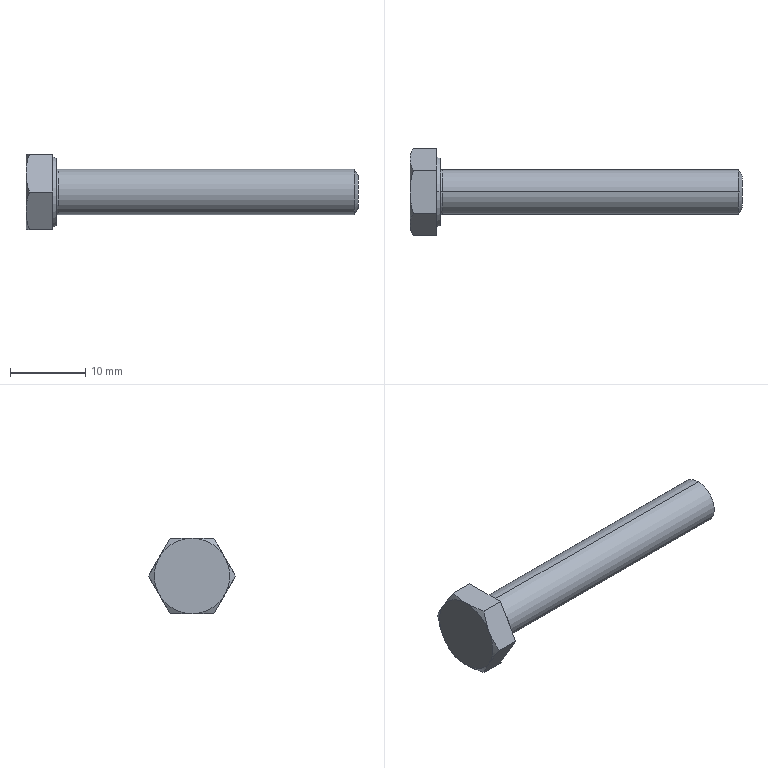Part | SolidWorks | features RevCut 3, Extrusion 1, Fillet 1, LPattern 1, Revolution 1 | 1 solid | 24 faces | box 44 x 11.547 x 10 mm | volume 1463 mm3 | cone 10 | plane 10 | torus 2 | cylinder 2 | commonest cylinder face diameters 6 x2
STEP:
#1=CARTESIAN_POINT('',(44.,0.,2.134));
#2=VERTEX_POINT('',#1);
#3=CARTESIAN_POINT('',(44.,0.,-2.134));
#4=VERTEX_POINT('',#3);
#5=CARTESIAN_POINT('',(44.,0.,0.));
#6=DIRECTION('',(-1.,0.,0.));
#7=DIRECTION('',(0.,0.,1.));
#8=AXIS2_PLACEMENT_3D('',#5,#6,#7);
#9=CIRCLE('',#8,2.134);
#10=EDGE_CURVE('',#2,#4,#9,.T.);
#11=ORIENTED_EDGE('',*,*,#10,.T.);
#12=CARTESIAN_POINT('',(43.5,0.,-3.));
#13=VERTEX_POINT('',#12);
#14=CARTESIAN_POINT('',(43.5,0.,-3.));
#15=DIRECTION('',(-0.5,0.,-0.866));
#16=VECTOR('',#15,1000.);
#17=LINE('',#14,#16);
#18=EDGE_CURVE('',#4,#13,#17,.T.);
#19=ORIENTED_EDGE('',*,*,#18,.T.);
#20=CARTESIAN_POINT('',(43.5,0.,3.));
#21=VERTEX_POINT('',#20);
#22=CARTESIAN_POINT('',(43.5,0.,0.));
#23=DIRECTION('',(-1.,0.,0.));
#24=DIRECTION('',(0.,0.,1.));
#25=AXIS2_PLACEMENT_3D('',#22,#23,#24);
#26=CIRCLE('',#25,3.);
#27=EDGE_CURVE('',#21,#13,#26,.T.);
#28=ORIENTED_EDGE('',*,*,#27,.F.);
#29=CARTESIAN_POINT('',(43.5,0.,3.));
#30=DIRECTION('',(-0.5,0.,0.866));
#31=VECTOR('',#30,1000.);
#32=LINE('',#29,#31);
#33=EDGE_CURVE('',#2,#21,#32,.T.);
#34=ORIENTED_EDGE('',*,*,#33,.F.);
#35=EDGE_LOOP('',(#11,#19,#28,#34));
#36=FACE_OUTER_BOUND('',#35,.T.);
#37=CARTESIAN_POINT('',(43.5,0.,0.));
#38=DIRECTION('',(-1.,0.,0.));
#39=DIRECTION('',(0.,0.,1.));
#40=AXIS2_PLACEMENT_3D('',#37,#38,#39);
#41=CONICAL_SURFACE('',#40,3.,1.047);
#42=ADVANCED_FACE('',(#36),#41,.T.);
#43=CARTESIAN_POINT('',(4.25,0.,3.));
#44=VERTEX_POINT('',#43);
#45=CARTESIAN_POINT('',(4.25,0.,-3.));
#46=VERTEX_POINT('',#45);
#47=CARTESIAN_POINT('',(4.25,0.,0.));
#48=DIRECTION('',(1.,0.,0.));
#49=DIRECTION('',(0.,0.,-1.));
#50=AXIS2_PLACEMENT_3D('',#47,#48,#49);
#51=CIRCLE('',#50,3.);
#52=EDGE_CURVE('',#44,#46,#51,.T.);
#53=ORIENTED_EDGE('',*,*,#52,.F.);
#54=CARTESIAN_POINT('',(4.,0.,3.25));
#55=VERTEX_POINT('',#54);
#56=CARTESIAN_POINT('',(4.25,0.,3.25));
#57=DIRECTION('',(0.,1.,0.));
#58=DIRECTION('',(0.,0.,1.));
#59=AXIS2_PLACEMENT_3D('',#56,#57,#58);
#60=CIRCLE('',#59,0.25);
#61=EDGE_CURVE('',#44,#55,#60,.T.);
#62=ORIENTED_EDGE('',*,*,#61,.T.);
#63=CARTESIAN_POINT('',(4.,0.,-3.25));
#64=VERTEX_POINT('',#63);
#65=CARTESIAN_POINT('',(4.,0.,0.));
#66=DIRECTION('',(-1.,0.,0.));
#67=DIRECTION('',(0.,0.,-1.));
#68=AXIS2_PLACEMENT_3D('',#65,#66,#67);
#69=CIRCLE('',#68,3.25);
#70=EDGE_CURVE('',#64,#55,#69,.T.);
#71=ORIENTED_EDGE('',*,*,#70,.F.);
#72=CARTESIAN_POINT('',(4.25,0.,-3.25));
#73=DIRECTION('',(0.,-1.,0.));
#74=DIRECTION('',(0.,0.,-1.));
#75=AXIS2_PLACEMENT_3D('',#72,#73,#74);
#76=CIRCLE('',#75,0.25);
#77=EDGE_CURVE('',#46,#64,#76,.T.);
#78=ORIENTED_EDGE('',*,*,#77,.F.);
#79=EDGE_LOOP('',(#53,#62,#71,#78));
#80=FACE_OUTER_BOUND('',#79,.T.);
#81=CARTESIAN_POINT('',(4.25,0.,0.));
#82=DIRECTION('',(1.,0.,0.));
#83=DIRECTION('',(0.,0.,-1.));
#84=AXIS2_PLACEMENT_3D('',#81,#82,#83);
#85=TOROIDAL_SURFACE('',#84,3.25,0.25);
#86=ADVANCED_FACE('',(#80),#85,.F.);
#87=CARTESIAN_POINT('',(4.,0.,4.44));
#88=VERTEX_POINT('',#87);
#89=CARTESIAN_POINT('',(4.,0.,-4.44));
#90=VERTEX_POINT('',#89);
#91=CARTESIAN_POINT('',(4.,0.,0.));
#92=DIRECTION('',(-1.,0.,0.));
#93=DIRECTION('',(0.,0.,1.));
#94=AXIS2_PLACEMENT_3D('',#91,#92,#93);
#95=CIRCLE('',#94,4.44);
#96=EDGE_CURVE('',#88,#90,#95,.T.);
#97=ORIENTED_EDGE('',*,*,#96,.T.);
#98=CARTESIAN_POINT('',(3.5,0.,-4.729));
#99=VERTEX_POINT('',#98);
#100=CARTESIAN_POINT('',(3.5,0.,-4.729));
#101=DIRECTION('',(-0.866,0.,-0.5));
#102=VECTOR('',#101,1000.);
#103=LINE('',#100,#102);
#104=EDGE_CURVE('',#90,#99,#103,.T.);
#105=ORIENTED_EDGE('',*,*,#104,.T.);
#106=CARTESIAN_POINT('',(3.5,0.,4.729));
#107=VERTEX_POINT('',#106);
#108=CARTESIAN_POINT('',(3.5,0.,0.));
#109=DIRECTION('',(-1.,0.,0.));
#110=DIRECTION('',(0.,0.,1.));
#111=AXIS2_PLACEMENT_3D('',#108,#109,#110);
#112=CIRCLE('',#111,4.729);
#113=EDGE_CURVE('',#107,#99,#112,.T.);
#114=ORIENTED_EDGE('',*,*,#113,.F.);
#115=CARTESIAN_POINT('',(3.5,0.,4.729));
#116=DIRECTION('',(-0.866,0.,0.5));
#117=VECTOR('',#116,1000.);
#118=LINE('',#115,#117);
#119=EDGE_CURVE('',#88,#107,#118,.T.);
#120=ORIENTED_EDGE('',*,*,#119,.F.);
#121=EDGE_LOOP('',(#97,#105,#114,#120));
#122=FACE_OUTER_BOUND('',#121,.T.);
#123=CARTESIAN_POINT('',(3.5,0.,0.));
#124=DIRECTION('',(-1.,0.,0.));
#125=DIRECTION('',(0.,0.,1.));
#126=AXIS2_PLACEMENT_3D('',#123,#124,#125);
#127=CONICAL_SURFACE('',#126,4.729,0.5236);
#128=ADVANCED_FACE('',(#122),#127,.T.);
#129=ORIENTED_EDGE('',*,*,#27,.T.);
#130=CARTESIAN_POINT('',(0.,0.,-3.));
#131=DIRECTION('',(-1.,0.,0.));
#132=VECTOR('',#131,1000.);
#133=LINE('',#130,#132);
#134=EDGE_CURVE('',#13,#46,#133,.T.);
#135=ORIENTED_EDGE('',*,*,#134,.T.);
#136=CARTESIAN_POINT('',(4.25,0.,0.));
#137=DIRECTION('',(1.,0.,0.));
#138=DIRECTION('',(0.,0.,-1.));
#139=AXIS2_PLACEMENT_3D('',#136,#137,#138);
#140=CIRCLE('',#139,3.);
#141=EDGE_CURVE('',#46,#44,#140,.T.);
#142=ORIENTED_EDGE('',*,*,#141,.T.);
#143=CARTESIAN_POINT('',(0.,0.,3.));
#144=DIRECTION('',(-1.,0.,0.));
#145=VECTOR('',#144,1000.);
#146=LINE('',#143,#145);
#147=EDGE_CURVE('',#21,#44,#146,.T.);
#148=ORIENTED_EDGE('',*,*,#147,.F.);
#149=EDGE_LOOP('',(#129,#135,#142,#148));
#150=FACE_OUTER_BOUND('',#149,.T.);
#151=CARTESIAN_POINT('',(0.,0.,0.));
#152=DIRECTION('',(-1.,0.,0.));
#153=DIRECTION('',(0.,0.,1.));
#154=AXIS2_PLACEMENT_3D('',#151,#152,#153);
#155=CYLINDRICAL_SURFACE('',#154,3.);
#156=ADVANCED_FACE('',(#150),#155,.T.);
#157=ORIENTED_EDGE('',*,*,#134,.F.);
#158=CARTESIAN_POINT('',(43.5,0.,0.));
#159=DIRECTION('',(-1.,0.,0.));
#160=DIRECTION('',(0.,0.,1.));
#161=AXIS2_PLACEMENT_3D('',#158,#159,#160);
#162=CIRCLE('',#161,3.);
#163=EDGE_CURVE('',#13,#21,#162,.T.);
#164=ORIENTED_EDGE('',*,*,#163,.T.);
#165=ORIENTED_EDGE('',*,*,#147,.T.);
#166=ORIENTED_EDGE('',*,*,#52,.T.);
#167=EDGE_LOOP('',(#157,#164,#165,#166));
#168=FACE_OUTER_BOUND('',#167,.T.);
#169=CARTESIAN_POINT('',(0.,0.,0.));
#170=DIRECTION('',(-1.,0.,0.));
#171=DIRECTION('',(0.,0.,1.));
#172=AXIS2_PLACEMENT_3D('',#169,#170,#171);
#173=CYLINDRICAL_SURFACE('',#172,3.);
#174=ADVANCED_FACE('',(#168),#173,.T.);
#175=CARTESIAN_POINT('',(3.5,2.887,-5.));
#176=VERTEX_POINT('',#175);
#177=CARTESIAN_POINT('',(3.5,5.774,0.));
#178=VERTEX_POINT('',#177);
#179=CARTESIAN_POINT('',(3.5,2.887,-5.));
#180=DIRECTION('',(0.,0.5,0.866));
#181=VECTOR('',#180,1000.);
#182=LINE('',#179,#181);
#183=EDGE_CURVE('',#176,#178,#182,.T.);
#184=ORIENTED_EDGE('',*,*,#183,.F.);
#185=CARTESIAN_POINT('',(0.4466,2.887,-5.));
#186=VERTEX_POINT('',#185);
#187=CARTESIAN_POINT('',(4.,2.887,-5.));
#188=DIRECTION('',(-1.,0.,0.));
#189=VECTOR('',#188,1000.);
#190=LINE('',#187,#189);
#191=EDGE_CURVE('',#176,#186,#190,.T.);
#192=ORIENTED_EDGE('',*,*,#191,.T.);
#193=CARTESIAN_POINT('',(0.,4.33,-2.5));
#194=VERTEX_POINT('',#193);
#195=CARTESIAN_POINT('',(0.,4.33,-2.5));
#196=CARTESIAN_POINT('',(0.,4.208,-2.712));
#197=CARTESIAN_POINT('',(0.01056,4.085,-2.925));
#198=CARTESIAN_POINT('',(0.0514,3.841,-3.347));
#199=CARTESIAN_POINT('',(0.08166,3.72,-3.556));
#200=CARTESIAN_POINT('',(0.1983,3.36,-4.181));
#201=CARTESIAN_POINT('',(0.3106,3.122,-4.592));
#202=CARTESIAN_POINT('',(0.4466,2.887,-5.));
#203=B_SPLINE_CURVE_WITH_KNOTS('',3,(#195,#196,#197,#198,#199,#200,#201,#202),.UNSPECIFIED.,.F.,.F.,(4,2,2,4),(0.002921,0.003649,0.004376,0.005831),.UNSPECIFIED.);
#204=EDGE_CURVE('',#194,#186,#203,.T.);
#205=ORIENTED_EDGE('',*,*,#204,.F.);
#206=CARTESIAN_POINT('',(0.4466,5.774,0.));
#207=VERTEX_POINT('',#206);
#208=CARTESIAN_POINT('',(0.4466,5.774,0.));
#209=CARTESIAN_POINT('',(0.1739,5.301,-0.8179));
#210=CARTESIAN_POINT('',(0.,4.822,-1.648));
#211=CARTESIAN_POINT('',(0.,4.33,-2.5));
#212=B_SPLINE_CURVE_WITH_KNOTS('',3,(#208,#209,#210,#211),.UNSPECIFIED.,.F.,.F.,(4,4),(0.000000238,0.002921),.UNSPECIFIED.);
#213=EDGE_CURVE('',#207,#194,#212,.T.);
#214=ORIENTED_EDGE('',*,*,#213,.F.);
#215=CARTESIAN_POINT('',(4.,5.774,0.));
#216=DIRECTION('',(-1.,0.,0.));
#217=VECTOR('',#216,1000.);
#218=LINE('',#215,#217);
#219=EDGE_CURVE('',#178,#207,#218,.T.);
#220=ORIENTED_EDGE('',*,*,#219,.F.);
#221=EDGE_LOOP('',(#184,#192,#205,#214,#220));
#222=FACE_OUTER_BOUND('',#221,.T.);
#223=CARTESIAN_POINT('',(4.,2.887,-5.));
#224=DIRECTION('',(0.,-0.866,0.5));
#225=DIRECTION('',(0.,-0.5,-0.866));
#226=AXIS2_PLACEMENT_3D('',#223,#224,#225);
#227=PLANE('',#226);
#228=ADVANCED_FACE('',(#222),#227,.F.);
#229=CARTESIAN_POINT('',(3.5,2.887,5.));
#230=VERTEX_POINT('',#229);
#231=CARTESIAN_POINT('',(3.5,5.774,0.));
#232=DIRECTION('',(0.,-0.5,0.866));
#233=VECTOR('',#232,1000.);
#234=LINE('',#231,#233);
#235=EDGE_CURVE('',#178,#230,#234,.T.);
#236=ORIENTED_EDGE('',*,*,#235,.F.);
#237=ORIENTED_EDGE('',*,*,#219,.T.);
#238=CARTESIAN_POINT('',(0.,4.33,2.5));
#239=VERTEX_POINT('',#238);
#240=CARTESIAN_POINT('',(0.,4.33,2.5));
#241=CARTESIAN_POINT('',(0.,4.453,2.288));
#242=CARTESIAN_POINT('',(0.01056,4.576,2.075));
#243=CARTESIAN_POINT('',(0.0514,4.819,1.653));
#244=CARTESIAN_POINT('',(0.08166,4.94,1.444));
#245=CARTESIAN_POINT('',(0.1983,5.3,0.8193));
#246=CARTESIAN_POINT('',(0.3106,5.538,0.4079));
#247=CARTESIAN_POINT('',(0.4466,5.774,0.));
#248=B_SPLINE_CURVE_WITH_KNOTS('',3,(#240,#241,#242,#243,#244,#245,#246,#247),.UNSPECIFIED.,.F.,.F.,(4,2,2,4),(0.002921,0.003649,0.004376,0.005831),.UNSPECIFIED.);
#249=EDGE_CURVE('',#239,#207,#248,.T.);
#250=ORIENTED_EDGE('',*,*,#249,.F.);
#251=CARTESIAN_POINT('',(0.4466,2.887,5.));
#252=VERTEX_POINT('',#251);
#253=CARTESIAN_POINT('',(0.4466,2.887,5.));
#254=CARTESIAN_POINT('',(0.1739,3.359,4.182));
#255=CARTESIAN_POINT('',(0.,3.838,3.352));
#256=CARTESIAN_POINT('',(0.,4.33,2.5));
#257=B_SPLINE_CURVE_WITH_KNOTS('',3,(#253,#254,#255,#256),.UNSPECIFIED.,.F.,.F.,(4,4),(0.000000238,0.002921),.UNSPECIFIED.);
#258=EDGE_CURVE('',#252,#239,#257,.T.);
#259=ORIENTED_EDGE('',*,*,#258,.F.);
#260=CARTESIAN_POINT('',(4.,2.887,5.));
#261=DIRECTION('',(-1.,0.,0.));
#262=VECTOR('',#261,1000.);
#263=LINE('',#260,#262);
#264=EDGE_CURVE('',#230,#252,#263,.T.);
#265=ORIENTED_EDGE('',*,*,#264,.F.);
#266=EDGE_LOOP('',(#236,#237,#250,#259,#265));
#267=FACE_OUTER_BOUND('',#266,.T.);
#268=CARTESIAN_POINT('',(4.,5.774,0.));
#269=DIRECTION('',(0.,-0.866,-0.5));
#270=DIRECTION('',(0.,0.5,-0.866));
#271=AXIS2_PLACEMENT_3D('',#268,#269,#270);
#272=PLANE('',#271);
#273=ADVANCED_FACE('',(#267),#272,.F.);
#274=CARTESIAN_POINT('',(3.5,-2.887,5.));
#275=VERTEX_POINT('',#274);
#276=CARTESIAN_POINT('',(3.5,2.887,5.));
#277=DIRECTION('',(0.,-1.,0.));
#278=VECTOR('',#277,1000.);
#279=LINE('',#276,#278);
#280=EDGE_CURVE('',#230,#275,#279,.T.);
#281=ORIENTED_EDGE('',*,*,#280,.F.);
#282=ORIENTED_EDGE('',*,*,#264,.T.);
#283=CARTESIAN_POINT('',(0.,0.,5.));
#284=VERTEX_POINT('',#283);
#285=CARTESIAN_POINT('',(0.,0.,5.));
#286=CARTESIAN_POINT('',(0.,0.4887,5.));
#287=CARTESIAN_POINT('',(0.04321,0.9837,5.));
#288=CARTESIAN_POINT('',(0.1996,1.947,5.));
#289=CARTESIAN_POINT('',(0.3118,2.42,5.));
#290=CARTESIAN_POINT('',(0.4466,2.887,5.));
#291=B_SPLINE_CURVE_WITH_KNOTS('',3,(#285,#286,#287,#288,#289,#290),.UNSPECIFIED.,.F.,.F.,(4,2,4),(0.008262,0.009724,0.01119),.UNSPECIFIED.);
#292=EDGE_CURVE('',#284,#252,#291,.T.);
#293=ORIENTED_EDGE('',*,*,#292,.F.);
#294=CARTESIAN_POINT('',(0.4466,-2.887,5.));
#295=VERTEX_POINT('',#294);
#296=CARTESIAN_POINT('',(0.4466,-2.887,5.));
#297=CARTESIAN_POINT('',(0.3109,-2.417,5.));
#298=CARTESIAN_POINT('',(0.1973,-1.936,5.));
#299=CARTESIAN_POINT('',(0.04202,-0.9731,5.));
#300=CARTESIAN_POINT('',(0.,-0.4884,5.));
#301=CARTESIAN_POINT('',(0.,0.,5.));
#302=B_SPLINE_CURVE_WITH_KNOTS('',3,(#296,#297,#298,#299,#300,#301),.UNSPECIFIED.,.F.,.F.,(4,2,4),(0.00534,0.006801,0.008262),.UNSPECIFIED.);
#303=EDGE_CURVE('',#295,#284,#302,.T.);
#304=ORIENTED_EDGE('',*,*,#303,.F.);
#305=CARTESIAN_POINT('',(4.,-2.887,5.));
#306=DIRECTION('',(-1.,0.,0.));
#307=VECTOR('',#306,1000.);
#308=LINE('',#305,#307);
#309=EDGE_CURVE('',#275,#295,#308,.T.);
#310=ORIENTED_EDGE('',*,*,#309,.F.);
#311=EDGE_LOOP('',(#281,#282,#293,#304,#310));
#312=FACE_OUTER_BOUND('',#311,.T.);
#313=CARTESIAN_POINT('',(4.,2.887,5.));
#314=DIRECTION('',(0.,0.,-1.));
#315=DIRECTION('',(0.,1.,0.));
#316=AXIS2_PLACEMENT_3D('',#313,#314,#315);
#317=PLANE('',#316);
#318=ADVANCED_FACE('',(#312),#317,.F.);
#319=CARTESIAN_POINT('',(3.5,-5.774,0.));
#320=VERTEX_POINT('',#319);
#321=CARTESIAN_POINT('',(3.5,-5.774,0.));
#322=DIRECTION('',(0.,-0.5,-0.866));
#323=VECTOR('',#322,1000.);
#324=LINE('',#321,#323);
#325=EDGE_CURVE('',#275,#320,#324,.T.);
#326=ORIENTED_EDGE('',*,*,#325,.F.);
#327=ORIENTED_EDGE('',*,*,#309,.T.);
#328=CARTESIAN_POINT('',(0.,-4.33,2.5));
#329=VERTEX_POINT('',#328);
#330=CARTESIAN_POINT('',(0.,-4.33,2.5));
#331=CARTESIAN_POINT('',(0.,-4.208,2.712));
#332=CARTESIAN_POINT('',(0.01056,-4.085,2.925));
#333=CARTESIAN_POINT('',(0.0514,-3.841,3.347));
#334=CARTESIAN_POINT('',(0.08166,-3.72,3.556));
#335=CARTESIAN_POINT('',(0.1983,-3.36,4.181));
#336=CARTESIAN_POINT('',(0.3106,-3.122,4.592));
#337=CARTESIAN_POINT('',(0.4466,-2.887,5.));
#338=B_SPLINE_CURVE_WITH_KNOTS('',3,(#330,#331,#332,#333,#334,#335,#336,#337),.UNSPECIFIED.,.F.,.F.,(4,2,2,4),(0.002921,0.003649,0.004376,0.005831),.UNSPECIFIED.);
#339=EDGE_CURVE('',#329,#295,#338,.T.);
#340=ORIENTED_EDGE('',*,*,#339,.F.);
#341=CARTESIAN_POINT('',(0.4466,-5.774,0.));
#342=VERTEX_POINT('',#341);
#343=CARTESIAN_POINT('',(0.4466,-5.774,0.));
#344=CARTESIAN_POINT('',(0.1739,-5.301,0.8179));
#345=CARTESIAN_POINT('',(0.,-4.822,1.648));
#346=CARTESIAN_POINT('',(0.,-4.33,2.5));
#347=B_SPLINE_CURVE_WITH_KNOTS('',3,(#343,#344,#345,#346),.UNSPECIFIED.,.F.,.F.,(4,4),(0.000000238,0.002921),.UNSPECIFIED.);
#348=EDGE_CURVE('',#342,#329,#347,.T.);
#349=ORIENTED_EDGE('',*,*,#348,.F.);
#350=CARTESIAN_POINT('',(4.,-5.774,0.));
#351=DIRECTION('',(-1.,0.,0.));
#352=VECTOR('',#351,1000.);
#353=LINE('',#350,#352);
#354=EDGE_CURVE('',#320,#342,#353,.T.);
#355=ORIENTED_EDGE('',*,*,#354,.F.);
#356=EDGE_LOOP('',(#326,#327,#340,#349,#355));
#357=FACE_OUTER_BOUND('',#356,.T.);
#358=CARTESIAN_POINT('',(4.,-5.774,0.));
#359=DIRECTION('',(0.,0.866,-0.5));
#360=DIRECTION('',(0.,0.5,0.866));
#361=AXIS2_PLACEMENT_3D('',#358,#359,#360);
#362=PLANE('',#361);
#363=ADVANCED_FACE('',(#357),#362,.F.);
#364=CARTESIAN_POINT('',(3.5,-2.887,-5.));
#365=VERTEX_POINT('',#364);
#366=CARTESIAN_POINT('',(3.5,-2.887,-5.));
#367=DIRECTION('',(0.,0.5,-0.866));
#368=VECTOR('',#367,1000.);
#369=LINE('',#366,#368);
#370=EDGE_CURVE('',#320,#365,#369,.T.);
#371=ORIENTED_EDGE('',*,*,#370,.F.);
#372=ORIENTED_EDGE('',*,*,#354,.T.);
#373=CARTESIAN_POINT('',(0.,-4.33,-2.5));
#374=VERTEX_POINT('',#373);
#375=CARTESIAN_POINT('',(0.,-4.33,-2.5));
#376=CARTESIAN_POINT('',(0.,-4.453,-2.288));
#377=CARTESIAN_POINT('',(0.01056,-4.576,-2.075));
#378=CARTESIAN_POINT('',(0.0514,-4.819,-1.653));
#379=CARTESIAN_POINT('',(0.08166,-4.94,-1.444));
#380=CARTESIAN_POINT('',(0.1983,-5.3,-0.8193));
#381=CARTESIAN_POINT('',(0.3106,-5.538,-0.4079));
#382=CARTESIAN_POINT('',(0.4466,-5.774,0.));
#383=B_SPLINE_CURVE_WITH_KNOTS('',3,(#375,#376,#377,#378,#379,#380,#381,#382),.UNSPECIFIED.,.F.,.F.,(4,2,2,4),(0.002921,0.003649,0.004376,0.005831),.UNSPECIFIED.);
#384=EDGE_CURVE('',#374,#342,#383,.T.);
#385=ORIENTED_EDGE('',*,*,#384,.F.);
#386=CARTESIAN_POINT('',(0.4466,-2.887,-5.));
#387=VERTEX_POINT('',#386);
#388=CARTESIAN_POINT('',(0.4466,-2.887,-5.));
#389=CARTESIAN_POINT('',(0.1739,-3.359,-4.182));
#390=CARTESIAN_POINT('',(0.,-3.838,-3.352));
#391=CARTESIAN_POINT('',(0.,-4.33,-2.5));
#392=B_SPLINE_CURVE_WITH_KNOTS('',3,(#388,#389,#390,#391),.UNSPECIFIED.,.F.,.F.,(4,4),(0.000000238,0.002921),.UNSPECIFIED.);
#393=EDGE_CURVE('',#387,#374,#392,.T.);
#394=ORIENTED_EDGE('',*,*,#393,.F.);
#395=CARTESIAN_POINT('',(4.,-2.887,-5.));
#396=DIRECTION('',(-1.,0.,0.));
#397=VECTOR('',#396,1000.);
#398=LINE('',#395,#397);
#399=EDGE_CURVE('',#365,#387,#398,.T.);
#400=ORIENTED_EDGE('',*,*,#399,.F.);
#401=EDGE_LOOP('',(#371,#372,#385,#394,#400));
#402=FACE_OUTER_BOUND('',#401,.T.);
#403=CARTESIAN_POINT('',(4.,-2.887,-5.));
#404=DIRECTION('',(0.,0.866,0.5));
#405=DIRECTION('',(0.,-0.5,0.866));
#406=AXIS2_PLACEMENT_3D('',#403,#404,#405);
#407=PLANE('',#406);
#408=ADVANCED_FACE('',(#402),#407,.F.);
#409=CARTESIAN_POINT('',(3.5,2.887,-5.));
#410=DIRECTION('',(0.,1.,0.));
#411=VECTOR('',#410,1000.);
#412=LINE('',#409,#411);
#413=EDGE_CURVE('',#365,#176,#412,.T.);
#414=ORIENTED_EDGE('',*,*,#413,.F.);
#415=ORIENTED_EDGE('',*,*,#399,.T.);
#416=CARTESIAN_POINT('',(0.,0.,-5.));
#417=VERTEX_POINT('',#416);
#418=CARTESIAN_POINT('',(0.,0.,-5.));
#419=CARTESIAN_POINT('',(0.,-0.4884,-5.));
#420=CARTESIAN_POINT('',(0.04202,-0.9731,-5.));
#421=CARTESIAN_POINT('',(0.1973,-1.936,-5.));
#422=CARTESIAN_POINT('',(0.3109,-2.417,-5.));
#423=CARTESIAN_POINT('',(0.4466,-2.887,-5.));
#424=B_SPLINE_CURVE_WITH_KNOTS('',3,(#418,#419,#420,#421,#422,#423),.UNSPECIFIED.,.F.,.F.,(4,2,4),(0.01799,0.01945,0.02091),.UNSPECIFIED.);
#425=EDGE_CURVE('',#417,#387,#424,.T.);
#426=ORIENTED_EDGE('',*,*,#425,.F.);
#427=CARTESIAN_POINT('',(0.4466,2.887,-5.));
#428=CARTESIAN_POINT('',(0.3118,2.42,-5.));
#429=CARTESIAN_POINT('',(0.1996,1.947,-5.));
#430=CARTESIAN_POINT('',(0.04321,0.9837,-5.));
#431=CARTESIAN_POINT('',(0.,0.4887,-5.));
#432=CARTESIAN_POINT('',(0.,0.,-5.));
#433=B_SPLINE_CURVE_WITH_KNOTS('',3,(#427,#428,#429,#430,#431,#432),.UNSPECIFIED.,.F.,.F.,(4,2,4),(0.01507,0.01653,0.01799),.UNSPECIFIED.);
#434=EDGE_CURVE('',#186,#417,#433,.T.);
#435=ORIENTED_EDGE('',*,*,#434,.F.);
#436=ORIENTED_EDGE('',*,*,#191,.F.);
#437=EDGE_LOOP('',(#414,#415,#426,#435,#436));
#438=FACE_OUTER_BOUND('',#437,.T.);
#439=CARTESIAN_POINT('',(4.,2.887,-5.));
#440=DIRECTION('',(0.,0.,1.));
#441=DIRECTION('',(0.,-1.,0.));
#442=AXIS2_PLACEMENT_3D('',#439,#440,#441);
#443=PLANE('',#442);
#444=ADVANCED_FACE('',(#438),#443,.F.);
#445=ORIENTED_EDGE('',*,*,#393,.T.);
#446=CARTESIAN_POINT('',(0.,0.,0.));
#447=DIRECTION('',(1.,0.,0.));
#448=DIRECTION('',(0.,0.,-1.));
#449=AXIS2_PLACEMENT_3D('',#446,#447,#448);
#450=CIRCLE('',#449,5.);
#451=EDGE_CURVE('',#374,#417,#450,.T.);
#452=ORIENTED_EDGE('',*,*,#451,.T.);
#453=ORIENTED_EDGE('',*,*,#425,.T.);
#454=EDGE_LOOP('',(#445,#452,#453));
#455=FACE_OUTER_BOUND('',#454,.T.);
#456=CARTESIAN_POINT('',(0.,0.,0.));
#457=DIRECTION('',(1.,0.,0.));
#458=DIRECTION('',(0.,0.,-1.));
#459=AXIS2_PLACEMENT_3D('',#456,#457,#458);
#460=CONICAL_SURFACE('',#459,5.,1.047);
#461=ADVANCED_FACE('',(#455),#460,.T.);
#462=ORIENTED_EDGE('',*,*,#348,.T.);
#463=CARTESIAN_POINT('',(0.,0.,0.));
#464=DIRECTION('',(1.,0.,0.));
#465=DIRECTION('',(0.,0.,-1.));
#466=AXIS2_PLACEMENT_3D('',#463,#464,#465);
#467=CIRCLE('',#466,5.);
#468=EDGE_CURVE('',#329,#374,#467,.T.);
#469=ORIENTED_EDGE('',*,*,#468,.T.);
#470=ORIENTED_EDGE('',*,*,#384,.T.);
#471=EDGE_LOOP('',(#462,#469,#470));
#472=FACE_OUTER_BOUND('',#471,.T.);
#473=CARTESIAN_POINT('',(0.,0.,0.));
#474=DIRECTION('',(1.,0.,0.));
#475=DIRECTION('',(0.,0.,-1.));
#476=AXIS2_PLACEMENT_3D('',#473,#474,#475);
#477=CONICAL_SURFACE('',#476,5.,1.047);
#478=ADVANCED_FACE('',(#472),#477,.T.);
#479=ORIENTED_EDGE('',*,*,#303,.T.);
#480=CARTESIAN_POINT('',(0.,0.,0.));
#481=DIRECTION('',(1.,0.,0.));
#482=DIRECTION('',(0.,0.,-1.));
#483=AXIS2_PLACEMENT_3D('',#480,#481,#482);
#484=CIRCLE('',#483,5.);
#485=EDGE_CURVE('',#284,#329,#484,.T.);
#486=ORIENTED_EDGE('',*,*,#485,.T.);
#487=ORIENTED_EDGE('',*,*,#339,.T.);
#488=EDGE_LOOP('',(#479,#486,#487));
#489=FACE_OUTER_BOUND('',#488,.T.);
#490=CARTESIAN_POINT('',(0.,0.,0.));
#491=DIRECTION('',(1.,0.,0.));
#492=DIRECTION('',(0.,0.,-1.));
#493=AXIS2_PLACEMENT_3D('',#490,#491,#492);
#494=CONICAL_SURFACE('',#493,5.,1.047);
#495=ADVANCED_FACE('',(#489),#494,.T.);
#496=ORIENTED_EDGE('',*,*,#292,.T.);
#497=ORIENTED_EDGE('',*,*,#258,.T.);
#498=CARTESIAN_POINT('',(0.,0.,0.));
#499=DIRECTION('',(-1.,0.,0.));
#500=DIRECTION('',(0.,0.,1.));
#501=AXIS2_PLACEMENT_3D('',#498,#499,#500);
#502=CIRCLE('',#501,5.);
#503=EDGE_CURVE('',#284,#239,#502,.T.);
#504=ORIENTED_EDGE('',*,*,#503,.F.);
#505=EDGE_LOOP('',(#496,#497,#504));
#506=FACE_OUTER_BOUND('',#505,.T.);
#507=CARTESIAN_POINT('',(0.,0.,0.));
#508=DIRECTION('',(1.,0.,0.));
#509=DIRECTION('',(0.,0.,-1.));
#510=AXIS2_PLACEMENT_3D('',#507,#508,#509);
#511=CONICAL_SURFACE('',#510,5.,1.047);
#512=ADVANCED_FACE('',(#506),#511,.T.);
#513=ORIENTED_EDGE('',*,*,#249,.T.);
#514=ORIENTED_EDGE('',*,*,#213,.T.);
#515=CARTESIAN_POINT('',(0.,0.,0.));
#516=DIRECTION('',(1.,0.,0.));
#517=DIRECTION('',(0.,0.,-1.));
#518=AXIS2_PLACEMENT_3D('',#515,#516,#517);
#519=CIRCLE('',#518,5.);
#520=EDGE_CURVE('',#194,#239,#519,.T.);
#521=ORIENTED_EDGE('',*,*,#520,.T.);
#522=EDGE_LOOP('',(#513,#514,#521));
#523=FACE_OUTER_BOUND('',#522,.T.);
#524=CARTESIAN_POINT('',(0.,0.,0.));
#525=DIRECTION('',(1.,0.,0.));
#526=DIRECTION('',(0.,0.,-1.));
#527=AXIS2_PLACEMENT_3D('',#524,#525,#526);
#528=CONICAL_SURFACE('',#527,5.,1.047);
#529=ADVANCED_FACE('',(#523),#528,.T.);
#530=ORIENTED_EDGE('',*,*,#204,.T.);
#531=ORIENTED_EDGE('',*,*,#434,.T.);
#532=CARTESIAN_POINT('',(0.,0.,0.));
#533=DIRECTION('',(1.,0.,0.));
#534=DIRECTION('',(0.,0.,-1.));
#535=AXIS2_PLACEMENT_3D('',#532,#533,#534);
#536=CIRCLE('',#535,5.);
#537=EDGE_CURVE('',#417,#194,#536,.T.);
#538=ORIENTED_EDGE('',*,*,#537,.T.);
#539=EDGE_LOOP('',(#530,#531,#538));
#540=FACE_OUTER_BOUND('',#539,.T.);
#541=CARTESIAN_POINT('',(0.,0.,0.));
#542=DIRECTION('',(1.,0.,0.));
#543=DIRECTION('',(0.,0.,-1.));
#544=AXIS2_PLACEMENT_3D('',#541,#542,#543);
#545=CONICAL_SURFACE('',#544,5.,1.047);
#546=ADVANCED_FACE('',(#540),#545,.T.);
#547=ORIENTED_EDGE('',*,*,#537,.F.);
#548=ORIENTED_EDGE('',*,*,#451,.F.);
#549=ORIENTED_EDGE('',*,*,#468,.F.);
#550=ORIENTED_EDGE('',*,*,#485,.F.);
#551=ORIENTED_EDGE('',*,*,#503,.T.);
#552=ORIENTED_EDGE('',*,*,#520,.F.);
#553=EDGE_LOOP('',(#547,#548,#549,#550,#551,#552));
#554=FACE_OUTER_BOUND('',#553,.T.);
#555=CARTESIAN_POINT('',(0.,0.,-10.));
#556=DIRECTION('',(1.,0.,0.));
#557=DIRECTION('',(0.,0.,-1.));
#558=AXIS2_PLACEMENT_3D('',#555,#556,#557);
#559=PLANE('',#558);
#560=ADVANCED_FACE('',(#554),#559,.F.);
#561=ORIENTED_EDGE('',*,*,#113,.T.);
#562=CARTESIAN_POINT('',(3.5,0.,0.));
#563=DIRECTION('',(-1.,0.,0.));
#564=DIRECTION('',(0.,0.,1.));
#565=AXIS2_PLACEMENT_3D('',#562,#563,#564);
#566=CIRCLE('',#565,4.729);
#567=EDGE_CURVE('',#99,#107,#566,.T.);
#568=ORIENTED_EDGE('',*,*,#567,.T.);
#569=EDGE_LOOP('',(#561,#568));
#570=FACE_BOUND('',#569,.T.);
#571=ORIENTED_EDGE('',*,*,#183,.T.);
#572=ORIENTED_EDGE('',*,*,#235,.T.);
#573=ORIENTED_EDGE('',*,*,#280,.T.);
#574=ORIENTED_EDGE('',*,*,#325,.T.);
#575=ORIENTED_EDGE('',*,*,#370,.T.);
#576=ORIENTED_EDGE('',*,*,#413,.T.);
#577=EDGE_LOOP('',(#571,#572,#573,#574,#575,#576));
#578=FACE_OUTER_BOUND('',#577,.T.);
#579=CARTESIAN_POINT('',(3.5,4.729,0.));
#580=DIRECTION('',(1.,0.,0.));
#581=DIRECTION('',(0.,0.,-1.));
#582=AXIS2_PLACEMENT_3D('',#579,#580,#581);
#583=PLANE('',#582);
#584=ADVANCED_FACE('',(#570,#578),#583,.T.);
#585=ORIENTED_EDGE('',*,*,#104,.F.);
#586=CARTESIAN_POINT('',(4.,0.,0.));
#587=DIRECTION('',(-1.,0.,0.));
#588=DIRECTION('',(0.,0.,1.));
#589=AXIS2_PLACEMENT_3D('',#586,#587,#588);
#590=CIRCLE('',#589,4.44);
#591=EDGE_CURVE('',#90,#88,#590,.T.);
#592=ORIENTED_EDGE('',*,*,#591,.T.);
#593=ORIENTED_EDGE('',*,*,#119,.T.);
#594=ORIENTED_EDGE('',*,*,#567,.F.);
#595=EDGE_LOOP('',(#585,#592,#593,#594));
#596=FACE_OUTER_BOUND('',#595,.T.);
#597=CARTESIAN_POINT('',(3.5,0.,0.));
#598=DIRECTION('',(-1.,0.,0.));
#599=DIRECTION('',(0.,0.,1.));
#600=AXIS2_PLACEMENT_3D('',#597,#598,#599);
#601=CONICAL_SURFACE('',#600,4.729,0.5236);
#602=ADVANCED_FACE('',(#596),#601,.T.);
#603=ORIENTED_EDGE('',*,*,#70,.T.);
#604=CARTESIAN_POINT('',(4.,0.,0.));
#605=DIRECTION('',(-1.,0.,0.));
#606=DIRECTION('',(0.,0.,-1.));
#607=AXIS2_PLACEMENT_3D('',#604,#605,#606);
#608=CIRCLE('',#607,3.25);
#609=EDGE_CURVE('',#55,#64,#608,.T.);
#610=ORIENTED_EDGE('',*,*,#609,.T.);
#611=EDGE_LOOP('',(#603,#610));
#612=FACE_BOUND('',#611,.T.);
#613=ORIENTED_EDGE('',*,*,#96,.F.);
#614=ORIENTED_EDGE('',*,*,#591,.F.);
#615=EDGE_LOOP('',(#613,#614));
#616=FACE_OUTER_BOUND('',#615,.T.);
#617=CARTESIAN_POINT('',(4.,0.,-10.));
#618=DIRECTION('',(1.,0.,0.));
#619=DIRECTION('',(0.,0.,-1.));
#620=AXIS2_PLACEMENT_3D('',#617,#618,#619);
#621=PLANE('',#620);
#622=ADVANCED_FACE('',(#612,#616),#621,.T.);
#623=ORIENTED_EDGE('',*,*,#61,.F.);
#624=ORIENTED_EDGE('',*,*,#141,.F.);
#625=ORIENTED_EDGE('',*,*,#77,.T.);
#626=ORIENTED_EDGE('',*,*,#609,.F.);
#627=EDGE_LOOP('',(#623,#624,#625,#626));
#628=FACE_OUTER_BOUND('',#627,.T.);
#629=CARTESIAN_POINT('',(4.25,0.,0.));
#630=DIRECTION('',(1.,0.,0.));
#631=DIRECTION('',(0.,0.,-1.));
#632=AXIS2_PLACEMENT_3D('',#629,#630,#631);
#633=TOROIDAL_SURFACE('',#632,3.25,0.25);
#634=ADVANCED_FACE('',(#628),#633,.F.);
#635=ORIENTED_EDGE('',*,*,#18,.F.);
#636=CARTESIAN_POINT('',(44.,0.,0.));
#637=DIRECTION('',(-1.,0.,0.));
#638=DIRECTION('',(0.,0.,1.));
#639=AXIS2_PLACEMENT_3D('',#636,#637,#638);
#640=CIRCLE('',#639,2.134);
#641=EDGE_CURVE('',#4,#2,#640,.T.);
#642=ORIENTED_EDGE('',*,*,#641,.T.);
#643=ORIENTED_EDGE('',*,*,#33,.T.);
#644=ORIENTED_EDGE('',*,*,#163,.F.);
#645=EDGE_LOOP('',(#635,#642,#643,#644));
#646=FACE_OUTER_BOUND('',#645,.T.);
#647=CARTESIAN_POINT('',(43.5,0.,0.));
#648=DIRECTION('',(-1.,0.,0.));
#649=DIRECTION('',(0.,0.,1.));
#650=AXIS2_PLACEMENT_3D('',#647,#648,#649);
#651=CONICAL_SURFACE('',#650,3.,1.047);
#652=ADVANCED_FACE('',(#646),#651,.T.);
#653=ORIENTED_EDGE('',*,*,#10,.F.);
#654=ORIENTED_EDGE('',*,*,#641,.F.);
#655=EDGE_LOOP('',(#653,#654));
#656=FACE_OUTER_BOUND('',#655,.T.);
#657=CARTESIAN_POINT('',(44.,0.,0.));
#658=DIRECTION('',(-1.,0.,0.));
#659=DIRECTION('',(0.,0.,1.));
#660=AXIS2_PLACEMENT_3D('',#657,#658,#659);
#661=PLANE('',#660);
#662=ADVANCED_FACE('',(#656),#661,.F.);
#663=CLOSED_SHELL('',(#42,#86,#128,#156,#174,#228,#273,#318,#363,#408,#444,#461,#478,#495,#512,#529,#546,#560,#584,#602,#622,#634,#652,#662));
#664=MANIFOLD_SOLID_BREP('',#663);
#665=CARTESIAN_POINT('',(0.,0.,0.));
#666=DIRECTION('',(0.,0.,1.));
#667=DIRECTION('',(1.,0.,0.));
#668=AXIS2_PLACEMENT_3D('',#665,#666,#667);
#669=(LENGTH_UNIT()NAMED_UNIT(*)SI_UNIT(.MILLI.,.METRE.));
#670=UNCERTAINTY_MEASURE_WITH_UNIT(LENGTH_MEASURE(0.00001),#669,'','');
#671=(NAMED_UNIT(*)PLANE_ANGLE_UNIT()SI_UNIT($,.RADIAN.));
#672=(NAMED_UNIT(*)SI_UNIT($,.STERADIAN.)SOLID_ANGLE_UNIT());
#673=(GEOMETRIC_REPRESENTATION_CONTEXT(3)GLOBAL_UNCERTAINTY_ASSIGNED_CONTEXT((#670))GLOBAL_UNIT_ASSIGNED_CONTEXT((#669,#671,#672))REPRESENTATION_CONTEXT('',''));
#674=ADVANCED_BREP_SHAPE_REPRESENTATION('',(#664,#668),#673);